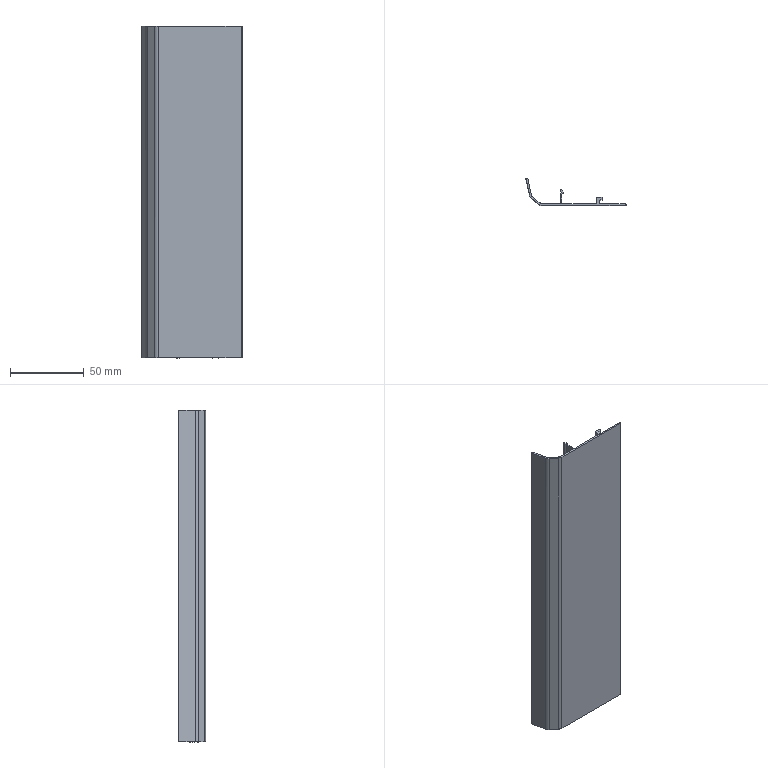Part | STEP file | 51E-01202JG10 | 1 solid | 49 faces | box 67.801 x 18.48 x 225 mm | volume 25716 mm3 | cylinder 28 | plane 21 | commonest cylinder face diameters 0.4 x11 0.6 x3 1 x3 1.2 x2 1.4 x2 4 x2